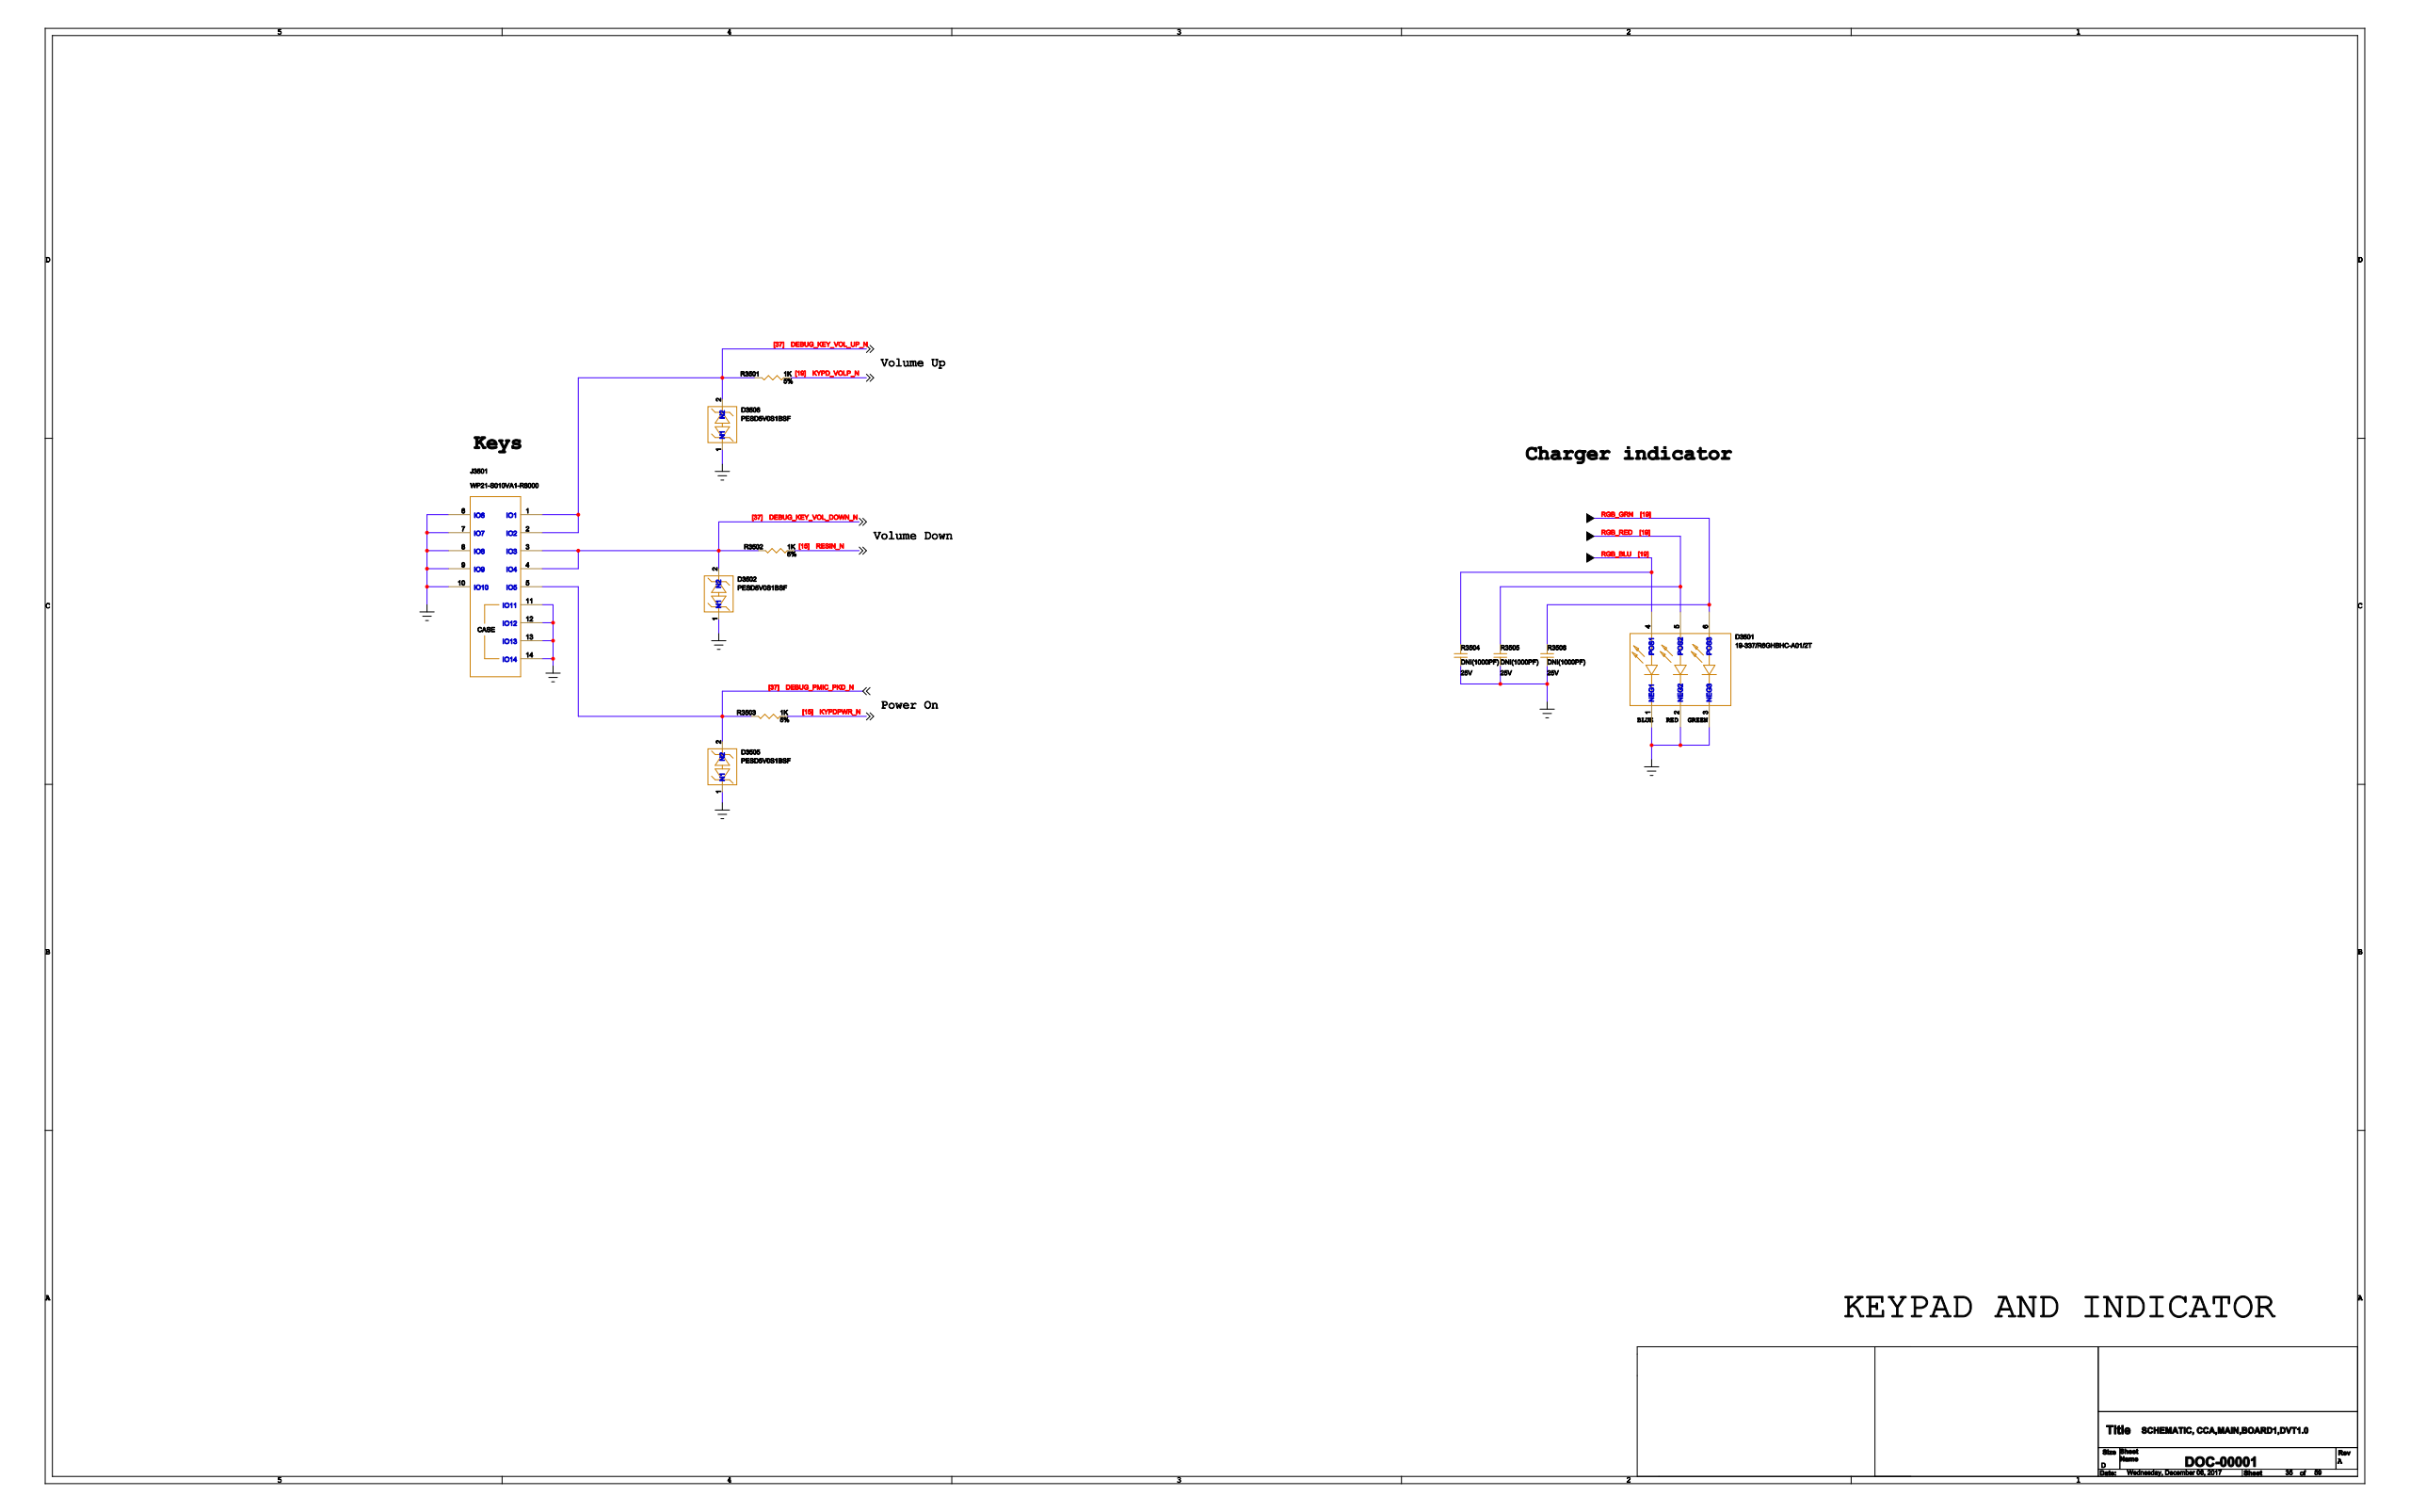Circuit board | KiCad | 1657 parts | 1365 nets | one sheet of the schematic
Parts on this sheet (reference | value | footprint):
D3501
D3502
D3505
D3506
J3501
R3501
R3502
R3503
R3504
R3505
R3506
Nets of these parts (net: part-pin ...):
GND: D3501-1 D3501-2 D3501-3 D3502-1 D3505-1 D3506-1 J3501-6 J3501-7 J3501-8 J3501-9 J3501-10 J3501-11 J3501-12 J3501-13 J3501-14 R3504-1 R3505-1 R3506-1
RGB_BLU: D3501-4 R3504-2
RGB_RED: D3501-5 R3505-2
RGB_GRN: D3501-6 R3506-2
BUG_PMIC_PKD_N: D3505-2 J3501-5 R3503-1
G_KEY_VOL_UP_N: D3506-2 J3501-1 J3501-2 R3501-1
KEY_VOL_DOWN_N: D3502-2 J3501-3 J3501-4 R3502-1
KYPDPWR_N: R3503-2
KYPD_VOLP_N: R3501-2
RESIN_N: R3502-2